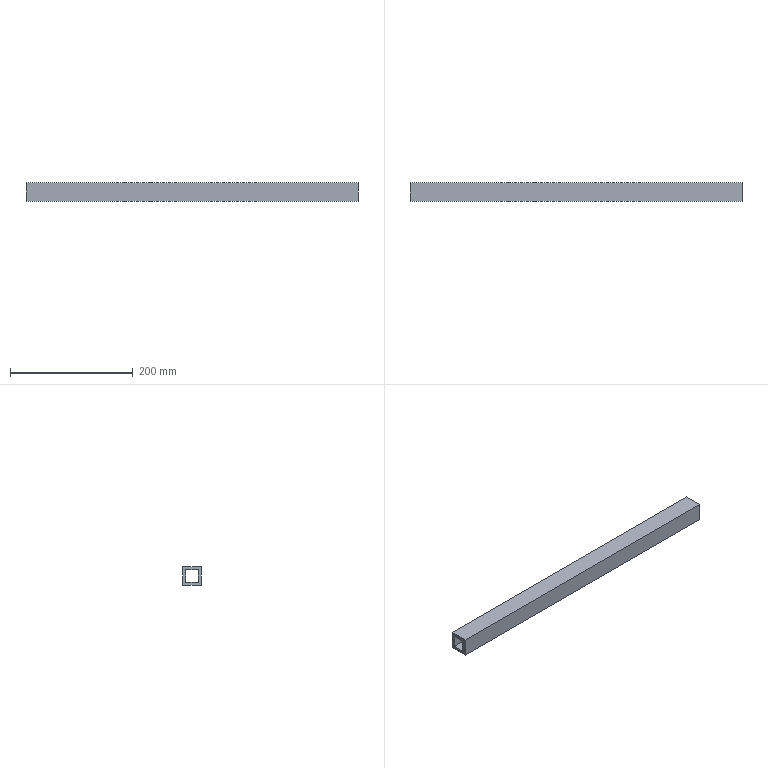Part | NX | features solid 2 | 1 solid | 10 faces | box 540 x 30 x 30 mm | volume 270000 mm3 | plane 10
STEP:
#1=CARTESIAN_POINT('',(175.,245.,-50.));
#2=VERTEX_POINT('',#1);
#3=CARTESIAN_POINT('',(175.,215.,-50.));
#4=VERTEX_POINT('',#3);
#5=CARTESIAN_POINT('',(175.,20.,-50.));
#6=DIRECTION('',(0.,1.,0.));
#7=VECTOR('',#6,1000.);
#8=LINE('',#5,#7);
#9=EDGE_CURVE('',#2,#4,#8,.F.);
#10=ORIENTED_EDGE('',*,*,#9,.T.);
#11=CARTESIAN_POINT('',(175.,215.,-20.));
#12=VERTEX_POINT('',#11);
#13=CARTESIAN_POINT('',(175.,215.,-20.));
#14=DIRECTION('',(0.,0.,-1.));
#15=VECTOR('',#14,1000.);
#16=LINE('',#13,#15);
#17=EDGE_CURVE('',#12,#4,#16,.T.);
#18=ORIENTED_EDGE('',*,*,#17,.F.);
#19=CARTESIAN_POINT('',(175.,245.,-20.));
#20=VERTEX_POINT('',#19);
#21=CARTESIAN_POINT('',(175.,245.,-20.));
#22=DIRECTION('',(0.,-1.,0.));
#23=VECTOR('',#22,1000.);
#24=LINE('',#21,#23);
#25=EDGE_CURVE('',#20,#12,#24,.T.);
#26=ORIENTED_EDGE('',*,*,#25,.F.);
#27=CARTESIAN_POINT('',(175.,245.,-20.));
#28=DIRECTION('',(0.,0.,1.));
#29=VECTOR('',#28,1000.);
#30=LINE('',#27,#29);
#31=EDGE_CURVE('',#20,#2,#30,.F.);
#32=ORIENTED_EDGE('',*,*,#31,.T.);
#33=EDGE_LOOP('',(#10,#18,#26,#32));
#34=FACE_BOUND('',#33,.T.);
#35=CARTESIAN_POINT('',(175.,240.,-25.));
#36=VERTEX_POINT('',#35);
#37=CARTESIAN_POINT('',(175.,240.,-45.));
#38=VERTEX_POINT('',#37);
#39=CARTESIAN_POINT('',(175.,240.,-20.));
#40=DIRECTION('',(0.,0.,1.));
#41=VECTOR('',#40,1000.);
#42=LINE('',#39,#41);
#43=EDGE_CURVE('',#36,#38,#42,.F.);
#44=ORIENTED_EDGE('',*,*,#43,.F.);
#45=CARTESIAN_POINT('',(175.,220.,-25.));
#46=VERTEX_POINT('',#45);
#47=CARTESIAN_POINT('',(175.,245.,-25.));
#48=DIRECTION('',(0.,-1.,0.));
#49=VECTOR('',#48,1000.);
#50=LINE('',#47,#49);
#51=EDGE_CURVE('',#36,#46,#50,.T.);
#52=ORIENTED_EDGE('',*,*,#51,.T.);
#53=CARTESIAN_POINT('',(175.,220.,-45.));
#54=VERTEX_POINT('',#53);
#55=CARTESIAN_POINT('',(175.,220.,-20.));
#56=DIRECTION('',(0.,0.,-1.));
#57=VECTOR('',#56,1000.);
#58=LINE('',#55,#57);
#59=EDGE_CURVE('',#46,#54,#58,.T.);
#60=ORIENTED_EDGE('',*,*,#59,.T.);
#61=CARTESIAN_POINT('',(175.,20.,-45.));
#62=DIRECTION('',(0.,1.,0.));
#63=VECTOR('',#62,1000.);
#64=LINE('',#61,#63);
#65=EDGE_CURVE('',#38,#54,#64,.F.);
#66=ORIENTED_EDGE('',*,*,#65,.F.);
#67=EDGE_LOOP('',(#44,#52,#60,#66));
#68=FACE_BOUND('',#67,.T.);
#69=CARTESIAN_POINT('',(175.,20.,-20.));
#70=DIRECTION('',(1.,0.,0.));
#71=DIRECTION('',(0.,0.,1.));
#72=AXIS2_PLACEMENT_3D('',#69,#70,#71);
#73=PLANE('',#72);
#74=ADVANCED_FACE('',(#34,#68),#73,.F.);
#75=CARTESIAN_POINT('',(715.,245.,-50.));
#76=VERTEX_POINT('',#75);
#77=CARTESIAN_POINT('',(715.,215.,-50.));
#78=VERTEX_POINT('',#77);
#79=CARTESIAN_POINT('',(715.,245.,-50.));
#80=DIRECTION('',(0.,-1.,0.));
#81=VECTOR('',#80,1000.);
#82=LINE('',#79,#81);
#83=EDGE_CURVE('',#76,#78,#82,.T.);
#84=ORIENTED_EDGE('',*,*,#83,.F.);
#85=CARTESIAN_POINT('',(715.,245.,-20.));
#86=VERTEX_POINT('',#85);
#87=CARTESIAN_POINT('',(715.,245.,-20.));
#88=DIRECTION('',(0.,0.,-1.));
#89=VECTOR('',#88,1000.);
#90=LINE('',#87,#89);
#91=EDGE_CURVE('',#86,#76,#90,.T.);
#92=ORIENTED_EDGE('',*,*,#91,.F.);
#93=CARTESIAN_POINT('',(715.,215.,-20.));
#94=VERTEX_POINT('',#93);
#95=CARTESIAN_POINT('',(715.,245.,-20.));
#96=DIRECTION('',(0.,1.,0.));
#97=VECTOR('',#96,1000.);
#98=LINE('',#95,#97);
#99=EDGE_CURVE('',#86,#94,#98,.F.);
#100=ORIENTED_EDGE('',*,*,#99,.T.);
#101=CARTESIAN_POINT('',(715.,215.,-20.));
#102=DIRECTION('',(0.,0.,1.));
#103=VECTOR('',#102,1000.);
#104=LINE('',#101,#103);
#105=EDGE_CURVE('',#94,#78,#104,.F.);
#106=ORIENTED_EDGE('',*,*,#105,.T.);
#107=EDGE_LOOP('',(#84,#92,#100,#106));
#108=FACE_BOUND('',#107,.T.);
#109=CARTESIAN_POINT('',(715.,240.,-45.));
#110=VERTEX_POINT('',#109);
#111=CARTESIAN_POINT('',(715.,220.,-45.));
#112=VERTEX_POINT('',#111);
#113=CARTESIAN_POINT('',(715.,245.,-45.));
#114=DIRECTION('',(0.,-1.,0.));
#115=VECTOR('',#114,1000.);
#116=LINE('',#113,#115);
#117=EDGE_CURVE('',#110,#112,#116,.T.);
#118=ORIENTED_EDGE('',*,*,#117,.T.);
#119=CARTESIAN_POINT('',(715.,220.,-25.));
#120=VERTEX_POINT('',#119);
#121=CARTESIAN_POINT('',(715.,220.,-20.));
#122=DIRECTION('',(0.,0.,1.));
#123=VECTOR('',#122,1000.);
#124=LINE('',#121,#123);
#125=EDGE_CURVE('',#120,#112,#124,.F.);
#126=ORIENTED_EDGE('',*,*,#125,.F.);
#127=CARTESIAN_POINT('',(715.,240.,-25.));
#128=VERTEX_POINT('',#127);
#129=CARTESIAN_POINT('',(715.,245.,-25.));
#130=DIRECTION('',(0.,1.,0.));
#131=VECTOR('',#130,1000.);
#132=LINE('',#129,#131);
#133=EDGE_CURVE('',#128,#120,#132,.F.);
#134=ORIENTED_EDGE('',*,*,#133,.F.);
#135=CARTESIAN_POINT('',(715.,240.,-20.));
#136=DIRECTION('',(0.,0.,-1.));
#137=VECTOR('',#136,1000.);
#138=LINE('',#135,#137);
#139=EDGE_CURVE('',#128,#110,#138,.T.);
#140=ORIENTED_EDGE('',*,*,#139,.T.);
#141=EDGE_LOOP('',(#118,#126,#134,#140));
#142=FACE_BOUND('',#141,.T.);
#143=CARTESIAN_POINT('',(715.,245.,-20.));
#144=DIRECTION('',(-1.,0.,0.));
#145=DIRECTION('',(0.,0.,-1.));
#146=AXIS2_PLACEMENT_3D('',#143,#144,#145);
#147=PLANE('',#146);
#148=ADVANCED_FACE('',(#108,#142),#147,.F.);
#149=CARTESIAN_POINT('',(205.,215.,-20.));
#150=DIRECTION('',(1.,0.,0.));
#151=VECTOR('',#150,1000.);
#152=LINE('',#149,#151);
#153=EDGE_CURVE('',#94,#12,#152,.F.);
#154=ORIENTED_EDGE('',*,*,#153,.F.);
#155=ORIENTED_EDGE('',*,*,#99,.F.);
#156=CARTESIAN_POINT('',(205.,245.,-20.));
#157=DIRECTION('',(1.,0.,0.));
#158=VECTOR('',#157,1000.);
#159=LINE('',#156,#158);
#160=EDGE_CURVE('',#86,#20,#159,.F.);
#161=ORIENTED_EDGE('',*,*,#160,.T.);
#162=ORIENTED_EDGE('',*,*,#25,.T.);
#163=EDGE_LOOP('',(#154,#155,#161,#162));
#164=FACE_BOUND('',#163,.T.);
#165=CARTESIAN_POINT('',(205.,245.,-20.));
#166=DIRECTION('',(0.,0.,1.));
#167=DIRECTION('',(0.,-1.,0.));
#168=AXIS2_PLACEMENT_3D('',#165,#166,#167);
#169=PLANE('',#168);
#170=ADVANCED_FACE('',(#164),#169,.T.);
#171=ORIENTED_EDGE('',*,*,#160,.F.);
#172=ORIENTED_EDGE('',*,*,#91,.T.);
#173=CARTESIAN_POINT('',(205.,245.,-50.));
#174=DIRECTION('',(1.,0.,0.));
#175=VECTOR('',#174,1000.);
#176=LINE('',#173,#175);
#177=EDGE_CURVE('',#76,#2,#176,.F.);
#178=ORIENTED_EDGE('',*,*,#177,.T.);
#179=ORIENTED_EDGE('',*,*,#31,.F.);
#180=EDGE_LOOP('',(#171,#172,#178,#179));
#181=FACE_BOUND('',#180,.T.);
#182=CARTESIAN_POINT('',(205.,245.,-20.));
#183=DIRECTION('',(0.,-1.,0.));
#184=DIRECTION('',(0.,0.,-1.));
#185=AXIS2_PLACEMENT_3D('',#182,#183,#184);
#186=PLANE('',#185);
#187=ADVANCED_FACE('',(#181),#186,.F.);
#188=ORIENTED_EDGE('',*,*,#177,.F.);
#189=ORIENTED_EDGE('',*,*,#83,.T.);
#190=CARTESIAN_POINT('',(205.,215.,-50.));
#191=DIRECTION('',(1.,0.,0.));
#192=VECTOR('',#191,1000.);
#193=LINE('',#190,#192);
#194=EDGE_CURVE('',#78,#4,#193,.F.);
#195=ORIENTED_EDGE('',*,*,#194,.T.);
#196=ORIENTED_EDGE('',*,*,#9,.F.);
#197=EDGE_LOOP('',(#188,#189,#195,#196));
#198=FACE_BOUND('',#197,.T.);
#199=CARTESIAN_POINT('',(205.,245.,-50.));
#200=DIRECTION('',(0.,0.,1.));
#201=DIRECTION('',(0.,-1.,0.));
#202=AXIS2_PLACEMENT_3D('',#199,#200,#201);
#203=PLANE('',#202);
#204=ADVANCED_FACE('',(#198),#203,.F.);
#205=ORIENTED_EDGE('',*,*,#105,.F.);
#206=ORIENTED_EDGE('',*,*,#153,.T.);
#207=ORIENTED_EDGE('',*,*,#17,.T.);
#208=ORIENTED_EDGE('',*,*,#194,.F.);
#209=EDGE_LOOP('',(#205,#206,#207,#208));
#210=FACE_BOUND('',#209,.T.);
#211=CARTESIAN_POINT('',(205.,215.,-20.));
#212=DIRECTION('',(0.,-1.,0.));
#213=DIRECTION('',(0.,0.,-1.));
#214=AXIS2_PLACEMENT_3D('',#211,#212,#213);
#215=PLANE('',#214);
#216=ADVANCED_FACE('',(#210),#215,.T.);
#217=CARTESIAN_POINT('',(205.,220.,-25.));
#218=DIRECTION('',(-1.,0.,0.));
#219=VECTOR('',#218,1000.);
#220=LINE('',#217,#219);
#221=EDGE_CURVE('',#120,#46,#220,.T.);
#222=ORIENTED_EDGE('',*,*,#221,.T.);
#223=ORIENTED_EDGE('',*,*,#51,.F.);
#224=CARTESIAN_POINT('',(205.,240.,-25.));
#225=DIRECTION('',(1.,0.,0.));
#226=VECTOR('',#225,1000.);
#227=LINE('',#224,#226);
#228=EDGE_CURVE('',#128,#36,#227,.F.);
#229=ORIENTED_EDGE('',*,*,#228,.F.);
#230=ORIENTED_EDGE('',*,*,#133,.T.);
#231=EDGE_LOOP('',(#222,#223,#229,#230));
#232=FACE_BOUND('',#231,.T.);
#233=CARTESIAN_POINT('',(205.,245.,-25.));
#234=DIRECTION('',(0.,0.,1.));
#235=DIRECTION('',(0.,-1.,0.));
#236=AXIS2_PLACEMENT_3D('',#233,#234,#235);
#237=PLANE('',#236);
#238=ADVANCED_FACE('',(#232),#237,.F.);
#239=ORIENTED_EDGE('',*,*,#228,.T.);
#240=ORIENTED_EDGE('',*,*,#43,.T.);
#241=CARTESIAN_POINT('',(205.,240.,-45.));
#242=DIRECTION('',(-1.,0.,0.));
#243=VECTOR('',#242,1000.);
#244=LINE('',#241,#243);
#245=EDGE_CURVE('',#110,#38,#244,.T.);
#246=ORIENTED_EDGE('',*,*,#245,.F.);
#247=ORIENTED_EDGE('',*,*,#139,.F.);
#248=EDGE_LOOP('',(#239,#240,#246,#247));
#249=FACE_BOUND('',#248,.T.);
#250=CARTESIAN_POINT('',(205.,240.,-20.));
#251=DIRECTION('',(0.,-1.,0.));
#252=DIRECTION('',(0.,0.,-1.));
#253=AXIS2_PLACEMENT_3D('',#250,#251,#252);
#254=PLANE('',#253);
#255=ADVANCED_FACE('',(#249),#254,.T.);
#256=ORIENTED_EDGE('',*,*,#245,.T.);
#257=ORIENTED_EDGE('',*,*,#65,.T.);
#258=CARTESIAN_POINT('',(205.,220.,-45.));
#259=DIRECTION('',(1.,0.,0.));
#260=VECTOR('',#259,1000.);
#261=LINE('',#258,#260);
#262=EDGE_CURVE('',#112,#54,#261,.F.);
#263=ORIENTED_EDGE('',*,*,#262,.F.);
#264=ORIENTED_EDGE('',*,*,#117,.F.);
#265=EDGE_LOOP('',(#256,#257,#263,#264));
#266=FACE_BOUND('',#265,.T.);
#267=CARTESIAN_POINT('',(205.,245.,-45.));
#268=DIRECTION('',(0.,0.,1.));
#269=DIRECTION('',(0.,-1.,0.));
#270=AXIS2_PLACEMENT_3D('',#267,#268,#269);
#271=PLANE('',#270);
#272=ADVANCED_FACE('',(#266),#271,.T.);
#273=ORIENTED_EDGE('',*,*,#125,.T.);
#274=ORIENTED_EDGE('',*,*,#262,.T.);
#275=ORIENTED_EDGE('',*,*,#59,.F.);
#276=ORIENTED_EDGE('',*,*,#221,.F.);
#277=EDGE_LOOP('',(#273,#274,#275,#276));
#278=FACE_BOUND('',#277,.T.);
#279=CARTESIAN_POINT('',(205.,220.,-20.));
#280=DIRECTION('',(0.,-1.,0.));
#281=DIRECTION('',(0.,0.,-1.));
#282=AXIS2_PLACEMENT_3D('',#279,#280,#281);
#283=PLANE('',#282);
#284=ADVANCED_FACE('',(#278),#283,.F.);
#285=CLOSED_SHELL('',(#74,#148,#170,#187,#204,#216,#238,#255,#272,#284));
#286=MANIFOLD_SOLID_BREP('',#285);
#287=(LENGTH_UNIT()NAMED_UNIT(*)SI_UNIT(.MILLI.,.METRE.));
#288=UNCERTAINTY_MEASURE_WITH_UNIT(LENGTH_MEASURE(0.00001),#287,'','');
#289=(NAMED_UNIT(*)PLANE_ANGLE_UNIT()SI_UNIT($,.RADIAN.));
#290=(NAMED_UNIT(*)SI_UNIT($,.STERADIAN.)SOLID_ANGLE_UNIT());
#291=(GEOMETRIC_REPRESENTATION_CONTEXT(3)GLOBAL_UNCERTAINTY_ASSIGNED_CONTEXT((#288))GLOBAL_UNIT_ASSIGNED_CONTEXT((#287,#289,#290))REPRESENTATION_CONTEXT('',''));
#292=ADVANCED_BREP_SHAPE_REPRESENTATION('',(#286),#291);